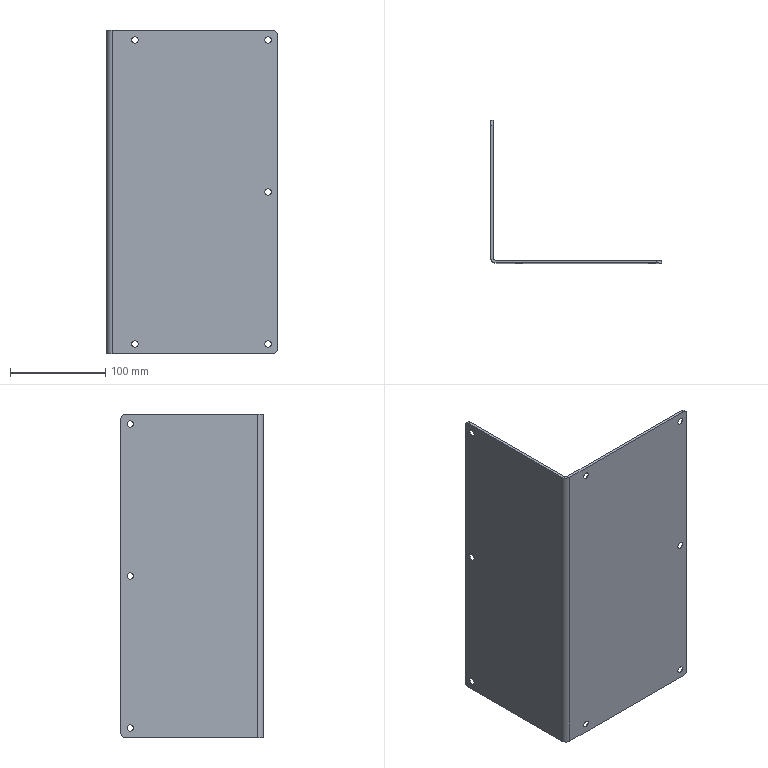Part | STEP file | PN_0001-12 Cover plate B | 1 solid | 30 faces | box 180 x 150 x 340 mm | volume 329639 mm3 | cone 16 | plane 8 | cylinder 6 | commonest cylinder face diameters 10 x4 6 x1 12 x1
STEP:
#1=CARTESIAN_POINT('',(0.,-10.,333.4));
#2=VERTEX_POINT('',#1);
#3=CARTESIAN_POINT('',(0.,-10.,326.6));
#4=VERTEX_POINT('',#3);
#5=CARTESIAN_POINT('',(0.,-10.,330.));
#6=DIRECTION('',(1.,0.,0.));
#7=DIRECTION('',(0.,1.,0.));
#8=AXIS2_PLACEMENT_3D('',#5,#6,#7);
#9=CIRCLE('',#8,3.4);
#10=EDGE_CURVE('',#2,#4,#9,.T.);
#11=ORIENTED_EDGE('',*,*,#10,.F.);
#12=CARTESIAN_POINT('',(3.,-10.,336.4));
#13=VERTEX_POINT('',#12);
#14=CARTESIAN_POINT('',(3.,-10.,336.4));
#15=DIRECTION('',(0.7071,0.,0.7071));
#16=VECTOR('',#15,1000.);
#17=LINE('',#14,#16);
#18=EDGE_CURVE('',#2,#13,#17,.T.);
#19=ORIENTED_EDGE('',*,*,#18,.T.);
#20=CARTESIAN_POINT('',(3.,-10.,323.6));
#21=VERTEX_POINT('',#20);
#22=CARTESIAN_POINT('',(3.,-10.,330.));
#23=DIRECTION('',(1.,0.,0.));
#24=DIRECTION('',(0.,0.,-1.));
#25=AXIS2_PLACEMENT_3D('',#22,#23,#24);
#26=CIRCLE('',#25,6.4);
#27=EDGE_CURVE('',#13,#21,#26,.T.);
#28=ORIENTED_EDGE('',*,*,#27,.T.);
#29=CARTESIAN_POINT('',(3.,-10.,323.6));
#30=DIRECTION('',(0.7071,0.,-0.7071));
#31=VECTOR('',#30,1000.);
#32=LINE('',#29,#31);
#33=EDGE_CURVE('',#4,#21,#32,.T.);
#34=ORIENTED_EDGE('',*,*,#33,.F.);
#35=EDGE_LOOP('',(#11,#19,#28,#34));
#36=FACE_OUTER_BOUND('',#35,.T.);
#37=CARTESIAN_POINT('',(3.,-10.,330.));
#38=DIRECTION('',(1.,0.,0.));
#39=DIRECTION('',(0.,0.,-1.));
#40=AXIS2_PLACEMENT_3D('',#37,#38,#39);
#41=CONICAL_SURFACE('',#40,6.4,0.7854);
#42=ADVANCED_FACE('',(#36),#41,.F.);
#43=CARTESIAN_POINT('',(0.,-10.,173.4));
#44=VERTEX_POINT('',#43);
#45=CARTESIAN_POINT('',(0.,-10.,166.6));
#46=VERTEX_POINT('',#45);
#47=CARTESIAN_POINT('',(0.,-10.,170.));
#48=DIRECTION('',(1.,0.,0.));
#49=DIRECTION('',(0.,1.,0.));
#50=AXIS2_PLACEMENT_3D('',#47,#48,#49);
#51=CIRCLE('',#50,3.4);
#52=EDGE_CURVE('',#44,#46,#51,.T.);
#53=ORIENTED_EDGE('',*,*,#52,.F.);
#54=CARTESIAN_POINT('',(3.,-10.,176.4));
#55=VERTEX_POINT('',#54);
#56=CARTESIAN_POINT('',(3.,-10.,176.4));
#57=DIRECTION('',(0.7071,0.,0.7071));
#58=VECTOR('',#57,1000.);
#59=LINE('',#56,#58);
#60=EDGE_CURVE('',#44,#55,#59,.T.);
#61=ORIENTED_EDGE('',*,*,#60,.T.);
#62=CARTESIAN_POINT('',(3.,-10.,163.6));
#63=VERTEX_POINT('',#62);
#64=CARTESIAN_POINT('',(3.,-10.,170.));
#65=DIRECTION('',(1.,0.,0.));
#66=DIRECTION('',(0.,0.,-1.));
#67=AXIS2_PLACEMENT_3D('',#64,#65,#66);
#68=CIRCLE('',#67,6.4);
#69=EDGE_CURVE('',#55,#63,#68,.T.);
#70=ORIENTED_EDGE('',*,*,#69,.T.);
#71=CARTESIAN_POINT('',(3.,-10.,163.6));
#72=DIRECTION('',(0.7071,0.,-0.7071));
#73=VECTOR('',#72,1000.);
#74=LINE('',#71,#73);
#75=EDGE_CURVE('',#46,#63,#74,.T.);
#76=ORIENTED_EDGE('',*,*,#75,.F.);
#77=EDGE_LOOP('',(#53,#61,#70,#76));
#78=FACE_OUTER_BOUND('',#77,.T.);
#79=CARTESIAN_POINT('',(3.,-10.,170.));
#80=DIRECTION('',(1.,0.,0.));
#81=DIRECTION('',(0.,0.,-1.));
#82=AXIS2_PLACEMENT_3D('',#79,#80,#81);
#83=CONICAL_SURFACE('',#82,6.4,0.7854);
#84=ADVANCED_FACE('',(#78),#83,.F.);
#85=CARTESIAN_POINT('',(0.,-10.,13.4));
#86=VERTEX_POINT('',#85);
#87=CARTESIAN_POINT('',(0.,-10.,6.6));
#88=VERTEX_POINT('',#87);
#89=CARTESIAN_POINT('',(0.,-10.,10.));
#90=DIRECTION('',(1.,0.,0.));
#91=DIRECTION('',(0.,1.,0.));
#92=AXIS2_PLACEMENT_3D('',#89,#90,#91);
#93=CIRCLE('',#92,3.4);
#94=EDGE_CURVE('',#86,#88,#93,.T.);
#95=ORIENTED_EDGE('',*,*,#94,.F.);
#96=CARTESIAN_POINT('',(3.,-10.,16.4));
#97=VERTEX_POINT('',#96);
#98=CARTESIAN_POINT('',(3.,-10.,16.4));
#99=DIRECTION('',(0.7071,0.,0.7071));
#100=VECTOR('',#99,1000.);
#101=LINE('',#98,#100);
#102=EDGE_CURVE('',#86,#97,#101,.T.);
#103=ORIENTED_EDGE('',*,*,#102,.T.);
#104=CARTESIAN_POINT('',(3.,-10.,3.6));
#105=VERTEX_POINT('',#104);
#106=CARTESIAN_POINT('',(3.,-10.,10.));
#107=DIRECTION('',(1.,0.,0.));
#108=DIRECTION('',(0.,0.,-1.));
#109=AXIS2_PLACEMENT_3D('',#106,#107,#108);
#110=CIRCLE('',#109,6.4);
#111=EDGE_CURVE('',#97,#105,#110,.T.);
#112=ORIENTED_EDGE('',*,*,#111,.T.);
#113=CARTESIAN_POINT('',(3.,-10.,3.6));
#114=DIRECTION('',(0.7071,0.,-0.7071));
#115=VECTOR('',#114,1000.);
#116=LINE('',#113,#115);
#117=EDGE_CURVE('',#88,#105,#116,.T.);
#118=ORIENTED_EDGE('',*,*,#117,.F.);
#119=EDGE_LOOP('',(#95,#103,#112,#118));
#120=FACE_OUTER_BOUND('',#119,.T.);
#121=CARTESIAN_POINT('',(3.,-10.,10.));
#122=DIRECTION('',(1.,0.,0.));
#123=DIRECTION('',(0.,0.,-1.));
#124=AXIS2_PLACEMENT_3D('',#121,#122,#123);
#125=CONICAL_SURFACE('',#124,6.4,0.7854);
#126=ADVANCED_FACE('',(#120),#125,.F.);
#127=CARTESIAN_POINT('',(30.,-150.,6.6));
#128=VERTEX_POINT('',#127);
#129=CARTESIAN_POINT('',(30.,-150.,13.4));
#130=VERTEX_POINT('',#129);
#131=CARTESIAN_POINT('',(30.,-150.,10.));
#132=DIRECTION('',(0.,1.,0.));
#133=DIRECTION('',(-1.,0.,0.));
#134=AXIS2_PLACEMENT_3D('',#131,#132,#133);
#135=CIRCLE('',#134,3.4);
#136=EDGE_CURVE('',#128,#130,#135,.T.);
#137=ORIENTED_EDGE('',*,*,#136,.F.);
#138=CARTESIAN_POINT('',(30.,-147.,3.6));
#139=VERTEX_POINT('',#138);
#140=CARTESIAN_POINT('',(30.,-147.,3.6));
#141=DIRECTION('',(0.,0.7071,-0.7071));
#142=VECTOR('',#141,1000.);
#143=LINE('',#140,#142);
#144=EDGE_CURVE('',#128,#139,#143,.T.);
#145=ORIENTED_EDGE('',*,*,#144,.T.);
#146=CARTESIAN_POINT('',(30.,-147.,16.4));
#147=VERTEX_POINT('',#146);
#148=CARTESIAN_POINT('',(30.,-147.,10.));
#149=DIRECTION('',(0.,1.,0.));
#150=DIRECTION('',(0.,0.,1.));
#151=AXIS2_PLACEMENT_3D('',#148,#149,#150);
#152=CIRCLE('',#151,6.4);
#153=EDGE_CURVE('',#139,#147,#152,.T.);
#154=ORIENTED_EDGE('',*,*,#153,.T.);
#155=CARTESIAN_POINT('',(30.,-147.,16.4));
#156=DIRECTION('',(0.,0.7071,0.7071));
#157=VECTOR('',#156,1000.);
#158=LINE('',#155,#157);
#159=EDGE_CURVE('',#130,#147,#158,.T.);
#160=ORIENTED_EDGE('',*,*,#159,.F.);
#161=EDGE_LOOP('',(#137,#145,#154,#160));
#162=FACE_OUTER_BOUND('',#161,.T.);
#163=CARTESIAN_POINT('',(30.,-147.,10.));
#164=DIRECTION('',(0.,1.,0.));
#165=DIRECTION('',(0.,0.,1.));
#166=AXIS2_PLACEMENT_3D('',#163,#164,#165);
#167=CONICAL_SURFACE('',#166,6.4,0.7854);
#168=ADVANCED_FACE('',(#162),#167,.F.);
#169=CARTESIAN_POINT('',(170.,-150.,6.6));
#170=VERTEX_POINT('',#169);
#171=CARTESIAN_POINT('',(170.,-150.,13.4));
#172=VERTEX_POINT('',#171);
#173=CARTESIAN_POINT('',(170.,-150.,10.));
#174=DIRECTION('',(0.,1.,0.));
#175=DIRECTION('',(-1.,0.,0.));
#176=AXIS2_PLACEMENT_3D('',#173,#174,#175);
#177=CIRCLE('',#176,3.4);
#178=EDGE_CURVE('',#170,#172,#177,.T.);
#179=ORIENTED_EDGE('',*,*,#178,.F.);
#180=CARTESIAN_POINT('',(170.,-147.,3.6));
#181=VERTEX_POINT('',#180);
#182=CARTESIAN_POINT('',(170.,-147.,3.6));
#183=DIRECTION('',(0.,0.7071,-0.7071));
#184=VECTOR('',#183,1000.);
#185=LINE('',#182,#184);
#186=EDGE_CURVE('',#170,#181,#185,.T.);
#187=ORIENTED_EDGE('',*,*,#186,.T.);
#188=CARTESIAN_POINT('',(170.,-147.,16.4));
#189=VERTEX_POINT('',#188);
#190=CARTESIAN_POINT('',(170.,-147.,10.));
#191=DIRECTION('',(0.,1.,0.));
#192=DIRECTION('',(0.,0.,1.));
#193=AXIS2_PLACEMENT_3D('',#190,#191,#192);
#194=CIRCLE('',#193,6.4);
#195=EDGE_CURVE('',#181,#189,#194,.T.);
#196=ORIENTED_EDGE('',*,*,#195,.T.);
#197=CARTESIAN_POINT('',(170.,-147.,16.4));
#198=DIRECTION('',(0.,0.7071,0.7071));
#199=VECTOR('',#198,1000.);
#200=LINE('',#197,#199);
#201=EDGE_CURVE('',#172,#189,#200,.T.);
#202=ORIENTED_EDGE('',*,*,#201,.F.);
#203=EDGE_LOOP('',(#179,#187,#196,#202));
#204=FACE_OUTER_BOUND('',#203,.T.);
#205=CARTESIAN_POINT('',(170.,-147.,10.));
#206=DIRECTION('',(0.,1.,0.));
#207=DIRECTION('',(0.,0.,1.));
#208=AXIS2_PLACEMENT_3D('',#205,#206,#207);
#209=CONICAL_SURFACE('',#208,6.4,0.7854);
#210=ADVANCED_FACE('',(#204),#209,.F.);
#211=CARTESIAN_POINT('',(170.,-150.,326.6));
#212=VERTEX_POINT('',#211);
#213=CARTESIAN_POINT('',(170.,-150.,333.4));
#214=VERTEX_POINT('',#213);
#215=CARTESIAN_POINT('',(170.,-150.,330.));
#216=DIRECTION('',(0.,1.,0.));
#217=DIRECTION('',(-1.,0.,0.));
#218=AXIS2_PLACEMENT_3D('',#215,#216,#217);
#219=CIRCLE('',#218,3.4);
#220=EDGE_CURVE('',#212,#214,#219,.T.);
#221=ORIENTED_EDGE('',*,*,#220,.F.);
#222=CARTESIAN_POINT('',(170.,-147.,323.6));
#223=VERTEX_POINT('',#222);
#224=CARTESIAN_POINT('',(170.,-147.,323.6));
#225=DIRECTION('',(0.,0.7071,-0.7071));
#226=VECTOR('',#225,1000.);
#227=LINE('',#224,#226);
#228=EDGE_CURVE('',#212,#223,#227,.T.);
#229=ORIENTED_EDGE('',*,*,#228,.T.);
#230=CARTESIAN_POINT('',(170.,-147.,336.4));
#231=VERTEX_POINT('',#230);
#232=CARTESIAN_POINT('',(170.,-147.,330.));
#233=DIRECTION('',(0.,1.,0.));
#234=DIRECTION('',(0.,0.,1.));
#235=AXIS2_PLACEMENT_3D('',#232,#233,#234);
#236=CIRCLE('',#235,6.4);
#237=EDGE_CURVE('',#223,#231,#236,.T.);
#238=ORIENTED_EDGE('',*,*,#237,.T.);
#239=CARTESIAN_POINT('',(170.,-147.,336.4));
#240=DIRECTION('',(0.,0.7071,0.7071));
#241=VECTOR('',#240,1000.);
#242=LINE('',#239,#241);
#243=EDGE_CURVE('',#214,#231,#242,.T.);
#244=ORIENTED_EDGE('',*,*,#243,.F.);
#245=EDGE_LOOP('',(#221,#229,#238,#244));
#246=FACE_OUTER_BOUND('',#245,.T.);
#247=CARTESIAN_POINT('',(170.,-147.,330.));
#248=DIRECTION('',(0.,1.,0.));
#249=DIRECTION('',(0.,0.,1.));
#250=AXIS2_PLACEMENT_3D('',#247,#248,#249);
#251=CONICAL_SURFACE('',#250,6.4,0.7854);
#252=ADVANCED_FACE('',(#246),#251,.F.);
#253=CARTESIAN_POINT('',(30.,-150.,326.6));
#254=VERTEX_POINT('',#253);
#255=CARTESIAN_POINT('',(30.,-150.,333.4));
#256=VERTEX_POINT('',#255);
#257=CARTESIAN_POINT('',(30.,-150.,330.));
#258=DIRECTION('',(0.,1.,0.));
#259=DIRECTION('',(-1.,0.,0.));
#260=AXIS2_PLACEMENT_3D('',#257,#258,#259);
#261=CIRCLE('',#260,3.4);
#262=EDGE_CURVE('',#254,#256,#261,.T.);
#263=ORIENTED_EDGE('',*,*,#262,.F.);
#264=CARTESIAN_POINT('',(30.,-147.,323.6));
#265=VERTEX_POINT('',#264);
#266=CARTESIAN_POINT('',(30.,-147.,323.6));
#267=DIRECTION('',(0.,0.7071,-0.7071));
#268=VECTOR('',#267,1000.);
#269=LINE('',#266,#268);
#270=EDGE_CURVE('',#254,#265,#269,.T.);
#271=ORIENTED_EDGE('',*,*,#270,.T.);
#272=CARTESIAN_POINT('',(30.,-147.,336.4));
#273=VERTEX_POINT('',#272);
#274=CARTESIAN_POINT('',(30.,-147.,330.));
#275=DIRECTION('',(0.,1.,0.));
#276=DIRECTION('',(0.,0.,1.));
#277=AXIS2_PLACEMENT_3D('',#274,#275,#276);
#278=CIRCLE('',#277,6.4);
#279=EDGE_CURVE('',#265,#273,#278,.T.);
#280=ORIENTED_EDGE('',*,*,#279,.T.);
#281=CARTESIAN_POINT('',(30.,-147.,336.4));
#282=DIRECTION('',(0.,0.7071,0.7071));
#283=VECTOR('',#282,1000.);
#284=LINE('',#281,#283);
#285=EDGE_CURVE('',#256,#273,#284,.T.);
#286=ORIENTED_EDGE('',*,*,#285,.F.);
#287=EDGE_LOOP('',(#263,#271,#280,#286));
#288=FACE_OUTER_BOUND('',#287,.T.);
#289=CARTESIAN_POINT('',(30.,-147.,330.));
#290=DIRECTION('',(0.,1.,0.));
#291=DIRECTION('',(0.,0.,1.));
#292=AXIS2_PLACEMENT_3D('',#289,#290,#291);
#293=CONICAL_SURFACE('',#292,6.4,0.7854);
#294=ADVANCED_FACE('',(#288),#293,.F.);
#295=CARTESIAN_POINT('',(170.,-150.,166.6));
#296=VERTEX_POINT('',#295);
#297=CARTESIAN_POINT('',(170.,-150.,173.4));
#298=VERTEX_POINT('',#297);
#299=CARTESIAN_POINT('',(170.,-150.,170.));
#300=DIRECTION('',(0.,1.,0.));
#301=DIRECTION('',(-1.,0.,0.));
#302=AXIS2_PLACEMENT_3D('',#299,#300,#301);
#303=CIRCLE('',#302,3.4);
#304=EDGE_CURVE('',#296,#298,#303,.T.);
#305=ORIENTED_EDGE('',*,*,#304,.F.);
#306=CARTESIAN_POINT('',(170.,-147.,163.6));
#307=VERTEX_POINT('',#306);
#308=CARTESIAN_POINT('',(170.,-147.,163.6));
#309=DIRECTION('',(0.,0.7071,-0.7071));
#310=VECTOR('',#309,1000.);
#311=LINE('',#308,#310);
#312=EDGE_CURVE('',#296,#307,#311,.T.);
#313=ORIENTED_EDGE('',*,*,#312,.T.);
#314=CARTESIAN_POINT('',(170.,-147.,176.4));
#315=VERTEX_POINT('',#314);
#316=CARTESIAN_POINT('',(170.,-147.,170.));
#317=DIRECTION('',(0.,1.,0.));
#318=DIRECTION('',(0.,0.,1.));
#319=AXIS2_PLACEMENT_3D('',#316,#317,#318);
#320=CIRCLE('',#319,6.4);
#321=EDGE_CURVE('',#307,#315,#320,.T.);
#322=ORIENTED_EDGE('',*,*,#321,.T.);
#323=CARTESIAN_POINT('',(170.,-147.,176.4));
#324=DIRECTION('',(0.,0.7071,0.7071));
#325=VECTOR('',#324,1000.);
#326=LINE('',#323,#325);
#327=EDGE_CURVE('',#298,#315,#326,.T.);
#328=ORIENTED_EDGE('',*,*,#327,.F.);
#329=EDGE_LOOP('',(#305,#313,#322,#328));
#330=FACE_OUTER_BOUND('',#329,.T.);
#331=CARTESIAN_POINT('',(170.,-147.,170.));
#332=DIRECTION('',(0.,1.,0.));
#333=DIRECTION('',(0.,0.,1.));
#334=AXIS2_PLACEMENT_3D('',#331,#332,#333);
#335=CONICAL_SURFACE('',#334,6.4,0.7854);
#336=ADVANCED_FACE('',(#330),#335,.F.);
#337=CARTESIAN_POINT('',(3.,-10.,330.));
#338=DIRECTION('',(1.,0.,0.));
#339=DIRECTION('',(0.,0.,-1.));
#340=AXIS2_PLACEMENT_3D('',#337,#338,#339);
#341=CIRCLE('',#340,6.4);
#342=EDGE_CURVE('',#21,#13,#341,.T.);
#343=ORIENTED_EDGE('',*,*,#342,.F.);
#344=ORIENTED_EDGE('',*,*,#27,.F.);
#345=EDGE_LOOP('',(#343,#344));
#346=FACE_BOUND('',#345,.T.);
#347=CARTESIAN_POINT('',(3.,-10.,170.));
#348=DIRECTION('',(1.,0.,0.));
#349=DIRECTION('',(0.,0.,-1.));
#350=AXIS2_PLACEMENT_3D('',#347,#348,#349);
#351=CIRCLE('',#350,6.4);
#352=EDGE_CURVE('',#63,#55,#351,.T.);
#353=ORIENTED_EDGE('',*,*,#352,.F.);
#354=ORIENTED_EDGE('',*,*,#69,.F.);
#355=EDGE_LOOP('',(#353,#354));
#356=FACE_BOUND('',#355,.T.);
#357=CARTESIAN_POINT('',(3.,-144.,0.));
#358=VERTEX_POINT('',#357);
#359=CARTESIAN_POINT('',(3.,-5.,0.));
#360=VERTEX_POINT('',#359);
#361=CARTESIAN_POINT('',(3.,-144.,0.));
#362=DIRECTION('',(0.,1.,0.));
#363=VECTOR('',#362,1000.);
#364=LINE('',#361,#363);
#365=EDGE_CURVE('',#358,#360,#364,.T.);
#366=ORIENTED_EDGE('',*,*,#365,.T.);
#367=CARTESIAN_POINT('',(3.,0.,5.));
#368=VERTEX_POINT('',#367);
#369=CARTESIAN_POINT('',(3.,-5.,5.));
#370=DIRECTION('',(1.,0.,0.));
#371=DIRECTION('',(0.,-1.,0.));
#372=AXIS2_PLACEMENT_3D('',#369,#370,#371);
#373=CIRCLE('',#372,5.);
#374=EDGE_CURVE('',#360,#368,#373,.T.);
#375=ORIENTED_EDGE('',*,*,#374,.T.);
#376=CARTESIAN_POINT('',(3.,0.,335.));
#377=VERTEX_POINT('',#376);
#378=CARTESIAN_POINT('',(3.,0.,340.));
#379=DIRECTION('',(0.,0.,-1.));
#380=VECTOR('',#379,1000.);
#381=LINE('',#378,#380);
#382=EDGE_CURVE('',#377,#368,#381,.T.);
#383=ORIENTED_EDGE('',*,*,#382,.F.);
#384=CARTESIAN_POINT('',(3.,-5.,340.));
#385=VERTEX_POINT('',#384);
#386=CARTESIAN_POINT('',(3.,-5.,335.));
#387=DIRECTION('',(1.,0.,0.));
#388=DIRECTION('',(0.,-1.,0.));
#389=AXIS2_PLACEMENT_3D('',#386,#387,#388);
#390=CIRCLE('',#389,5.);
#391=EDGE_CURVE('',#377,#385,#390,.T.);
#392=ORIENTED_EDGE('',*,*,#391,.T.);
#393=CARTESIAN_POINT('',(3.,-144.,340.));
#394=VERTEX_POINT('',#393);
#395=CARTESIAN_POINT('',(3.,-144.,340.));
#396=DIRECTION('',(0.,1.,0.));
#397=VECTOR('',#396,1000.);
#398=LINE('',#395,#397);
#399=EDGE_CURVE('',#394,#385,#398,.T.);
#400=ORIENTED_EDGE('',*,*,#399,.F.);
#401=CARTESIAN_POINT('',(3.,-144.,340.));
#402=DIRECTION('',(0.,0.,-1.));
#403=VECTOR('',#402,1000.);
#404=LINE('',#401,#403);
#405=EDGE_CURVE('',#394,#358,#404,.T.);
#406=ORIENTED_EDGE('',*,*,#405,.T.);
#407=EDGE_LOOP('',(#366,#375,#383,#392,#400,#406));
#408=FACE_OUTER_BOUND('',#407,.T.);
#409=CARTESIAN_POINT('',(3.,-10.,10.));
#410=DIRECTION('',(1.,0.,0.));
#411=DIRECTION('',(0.,0.,-1.));
#412=AXIS2_PLACEMENT_3D('',#409,#410,#411);
#413=CIRCLE('',#412,6.4);
#414=EDGE_CURVE('',#105,#97,#413,.T.);
#415=ORIENTED_EDGE('',*,*,#414,.F.);
#416=ORIENTED_EDGE('',*,*,#111,.F.);
#417=EDGE_LOOP('',(#415,#416));
#418=FACE_BOUND('',#417,.T.);
#419=CARTESIAN_POINT('',(3.,-144.,340.));
#420=DIRECTION('',(-1.,0.,0.));
#421=DIRECTION('',(0.,-1.,0.));
#422=AXIS2_PLACEMENT_3D('',#419,#420,#421);
#423=PLANE('',#422);
#424=ADVANCED_FACE('',(#346,#356,#408,#418),#423,.F.);
#425=ORIENTED_EDGE('',*,*,#382,.T.);
#426=CARTESIAN_POINT('',(0.,0.,5.));
#427=VERTEX_POINT('',#426);
#428=CARTESIAN_POINT('',(3.,0.,5.));
#429=DIRECTION('',(-1.,0.,0.));
#430=VECTOR('',#429,1000.);
#431=LINE('',#428,#430);
#432=EDGE_CURVE('',#368,#427,#431,.T.);
#433=ORIENTED_EDGE('',*,*,#432,.T.);
#434=CARTESIAN_POINT('',(0.,0.,335.));
#435=VERTEX_POINT('',#434);
#436=CARTESIAN_POINT('',(0.,0.,340.));
#437=DIRECTION('',(0.,0.,-1.));
#438=VECTOR('',#437,1000.);
#439=LINE('',#436,#438);
#440=EDGE_CURVE('',#435,#427,#439,.T.);
#441=ORIENTED_EDGE('',*,*,#440,.F.);
#442=CARTESIAN_POINT('',(3.,0.,335.));
#443=DIRECTION('',(1.,0.,0.));
#444=VECTOR('',#443,1000.);
#445=LINE('',#442,#444);
#446=EDGE_CURVE('',#435,#377,#445,.T.);
#447=ORIENTED_EDGE('',*,*,#446,.T.);
#448=EDGE_LOOP('',(#425,#433,#441,#447));
#449=FACE_OUTER_BOUND('',#448,.T.);
#450=CARTESIAN_POINT('',(3.,0.,340.));
#451=DIRECTION('',(0.,-1.,0.));
#452=DIRECTION('',(0.,0.,-1.));
#453=AXIS2_PLACEMENT_3D('',#450,#451,#452);
#454=PLANE('',#453);
#455=ADVANCED_FACE('',(#449),#454,.F.);
#456=CARTESIAN_POINT('',(0.,-10.,330.));
#457=DIRECTION('',(1.,0.,0.));
#458=DIRECTION('',(0.,1.,0.));
#459=AXIS2_PLACEMENT_3D('',#456,#457,#458);
#460=CIRCLE('',#459,3.4);
#461=EDGE_CURVE('',#4,#2,#460,.T.);
#462=ORIENTED_EDGE('',*,*,#461,.T.);
#463=ORIENTED_EDGE('',*,*,#10,.T.);
#464=EDGE_LOOP('',(#462,#463));
#465=FACE_BOUND('',#464,.T.);
#466=CARTESIAN_POINT('',(0.,-10.,170.));
#467=DIRECTION('',(1.,0.,0.));
#468=DIRECTION('',(0.,1.,0.));
#469=AXIS2_PLACEMENT_3D('',#466,#467,#468);
#470=CIRCLE('',#469,3.4);
#471=EDGE_CURVE('',#46,#44,#470,.T.);
#472=ORIENTED_EDGE('',*,*,#471,.T.);
#473=ORIENTED_EDGE('',*,*,#52,.T.);
#474=EDGE_LOOP('',(#472,#473));
#475=FACE_BOUND('',#474,.T.);
#476=CARTESIAN_POINT('',(0.,-10.,10.));
#477=DIRECTION('',(1.,0.,0.));
#478=DIRECTION('',(0.,1.,0.));
#479=AXIS2_PLACEMENT_3D('',#476,#477,#478);
#480=CIRCLE('',#479,3.4);
#481=EDGE_CURVE('',#88,#86,#480,.T.);
#482=ORIENTED_EDGE('',*,*,#481,.T.);
#483=ORIENTED_EDGE('',*,*,#94,.T.);
#484=EDGE_LOOP('',(#482,#483));
#485=FACE_BOUND('',#484,.T.);
#486=ORIENTED_EDGE('',*,*,#440,.T.);
#487=CARTESIAN_POINT('',(0.,-5.,0.));
#488=VERTEX_POINT('',#487);
#489=CARTESIAN_POINT('',(0.,-5.,5.));
#490=DIRECTION('',(-1.,0.,0.));
#491=DIRECTION('',(0.,1.,0.));
#492=AXIS2_PLACEMENT_3D('',#489,#490,#491);
#493=CIRCLE('',#492,5.);
#494=EDGE_CURVE('',#427,#488,#493,.T.);
#495=ORIENTED_EDGE('',*,*,#494,.T.);
#496=CARTESIAN_POINT('',(0.,-144.,0.));
#497=VERTEX_POINT('',#496);
#498=CARTESIAN_POINT('',(0.,0.,0.));
#499=DIRECTION('',(0.,-1.,0.));
#500=VECTOR('',#499,1000.);
#501=LINE('',#498,#500);
#502=EDGE_CURVE('',#488,#497,#501,.T.);
#503=ORIENTED_EDGE('',*,*,#502,.T.);
#504=CARTESIAN_POINT('',(0.,-144.,340.));
#505=VERTEX_POINT('',#504);
#506=CARTESIAN_POINT('',(0.,-144.,340.));
#507=DIRECTION('',(0.,0.,-1.));
#508=VECTOR('',#507,1000.);
#509=LINE('',#506,#508);
#510=EDGE_CURVE('',#505,#497,#509,.T.);
#511=ORIENTED_EDGE('',*,*,#510,.F.);
#512=CARTESIAN_POINT('',(0.,-5.,340.));
#513=VERTEX_POINT('',#512);
#514=CARTESIAN_POINT('',(0.,0.,340.));
#515=DIRECTION('',(0.,-1.,0.));
#516=VECTOR('',#515,1000.);
#517=LINE('',#514,#516);
#518=EDGE_CURVE('',#513,#505,#517,.T.);
#519=ORIENTED_EDGE('',*,*,#518,.F.);
#520=CARTESIAN_POINT('',(0.,-5.,335.));
#521=DIRECTION('',(-1.,0.,0.));
#522=DIRECTION('',(0.,1.,0.));
#523=AXIS2_PLACEMENT_3D('',#520,#521,#522);
#524=CIRCLE('',#523,5.);
#525=EDGE_CURVE('',#513,#435,#524,.T.);
#526=ORIENTED_EDGE('',*,*,#525,.T.);
#527=EDGE_LOOP('',(#486,#495,#503,#511,#519,#526));
#528=FACE_OUTER_BOUND('',#527,.T.);
#529=CARTESIAN_POINT('',(0.,0.,340.));
#530=DIRECTION('',(1.,0.,0.));
#531=DIRECTION('',(0.,1.,0.));
#532=AXIS2_PLACEMENT_3D('',#529,#530,#531);
#533=PLANE('',#532);
#534=ADVANCED_FACE('',(#465,#475,#485,#528),#533,.F.);
#535=CARTESIAN_POINT('',(6.,-150.,0.));
#536=VERTEX_POINT('',#535);
#537=CARTESIAN_POINT('',(6.,-144.,0.));
#538=DIRECTION('',(0.,0.,1.));
#539=DIRECTION('',(1.,0.,0.));
#540=AXIS2_PLACEMENT_3D('',#537,#538,#539);
#541=CIRCLE('',#540,6.);
#542=EDGE_CURVE('',#497,#536,#541,.T.);
#543=ORIENTED_EDGE('',*,*,#542,.T.);
#544=CARTESIAN_POINT('',(6.,-150.,340.));
#545=VERTEX_POINT('',#544);
#546=CARTESIAN_POINT('',(6.,-150.,340.));
#547=DIRECTION('',(0.,0.,-1.));
#548=VECTOR('',#547,1000.);
#549=LINE('',#546,#548);
#550=EDGE_CURVE('',#545,#536,#549,.T.);
#551=ORIENTED_EDGE('',*,*,#550,.F.);
#552=CARTESIAN_POINT('',(6.,-144.,340.));
#553=DIRECTION('',(0.,0.,1.));
#554=DIRECTION('',(1.,0.,0.));
#555=AXIS2_PLACEMENT_3D('',#552,#553,#554);
#556=CIRCLE('',#555,6.);
#557=EDGE_CURVE('',#505,#545,#556,.T.);
#558=ORIENTED_EDGE('',*,*,#557,.F.);
#559=ORIENTED_EDGE('',*,*,#510,.T.);
#560=EDGE_LOOP('',(#543,#551,#558,#559));
#561=FACE_OUTER_BOUND('',#560,.T.);
#562=CARTESIAN_POINT('',(6.,-144.,340.));
#563=DIRECTION('',(0.,0.,-1.));
#564=DIRECTION('',(-1.,0.,0.));
#565=AXIS2_PLACEMENT_3D('',#562,#563,#564);
#566=CYLINDRICAL_SURFACE('',#565,6.);
#567=ADVANCED_FACE('',(#561),#566,.T.);
#568=CARTESIAN_POINT('',(30.,-150.,10.));
#569=DIRECTION('',(0.,1.,0.));
#570=DIRECTION('',(-1.,0.,0.));
#571=AXIS2_PLACEMENT_3D('',#568,#569,#570);
#572=CIRCLE('',#571,3.4);
#573=EDGE_CURVE('',#130,#128,#572,.T.);
#574=ORIENTED_EDGE('',*,*,#573,.T.);
#575=ORIENTED_EDGE('',*,*,#136,.T.);
#576=EDGE_LOOP('',(#574,#575));
#577=FACE_BOUND('',#576,.T.);
#578=CARTESIAN_POINT('',(170.,-150.,10.));
#579=DIRECTION('',(0.,1.,0.));
#580=DIRECTION('',(-1.,0.,0.));
#581=AXIS2_PLACEMENT_3D('',#578,#579,#580);
#582=CIRCLE('',#581,3.4);
#583=EDGE_CURVE('',#172,#170,#582,.T.);
#584=ORIENTED_EDGE('',*,*,#583,.T.);
#585=ORIENTED_EDGE('',*,*,#178,.T.);
#586=EDGE_LOOP('',(#584,#585));
#587=FACE_BOUND('',#586,.T.);
#588=CARTESIAN_POINT('',(170.,-150.,330.));
#589=DIRECTION('',(0.,1.,0.));
#590=DIRECTION('',(-1.,0.,0.));
#591=AXIS2_PLACEMENT_3D('',#588,#589,#590);
#592=CIRCLE('',#591,3.4);
#593=EDGE_CURVE('',#214,#212,#592,.T.);
#594=ORIENTED_EDGE('',*,*,#593,.T.);
#595=ORIENTED_EDGE('',*,*,#220,.T.);
#596=EDGE_LOOP('',(#594,#595));
#597=FACE_BOUND('',#596,.T.);
#598=CARTESIAN_POINT('',(30.,-150.,330.));
#599=DIRECTION('',(0.,1.,0.));
#600=DIRECTION('',(-1.,0.,0.));
#601=AXIS2_PLACEMENT_3D('',#598,#599,#600);
#602=CIRCLE('',#601,3.4);
#603=EDGE_CURVE('',#256,#254,#602,.T.);
#604=ORIENTED_EDGE('',*,*,#603,.T.);
#605=ORIENTED_EDGE('',*,*,#262,.T.);
#606=EDGE_LOOP('',(#604,#605));
#607=FACE_BOUND('',#606,.T.);
#608=CARTESIAN_POINT('',(170.,-150.,170.));
#609=DIRECTION('',(0.,1.,0.));
#610=DIRECTION('',(-1.,0.,0.));
#611=AXIS2_PLACEMENT_3D('',#608,#609,#610);
#612=CIRCLE('',#611,3.4);
#613=EDGE_CURVE('',#298,#296,#612,.T.);
#614=ORIENTED_EDGE('',*,*,#613,.T.);
#615=ORIENTED_EDGE('',*,*,#304,.T.);
#616=EDGE_LOOP('',(#614,#615));
#617=FACE_BOUND('',#616,.T.);
#618=CARTESIAN_POINT('',(175.,-150.,0.));
#619=VERTEX_POINT('',#618);
#620=CARTESIAN_POINT('',(6.,-150.,0.));
#621=DIRECTION('',(1.,0.,0.));
#622=VECTOR('',#621,1000.);
#623=LINE('',#620,#622);
#624=EDGE_CURVE('',#536,#619,#623,.T.);
#625=ORIENTED_EDGE('',*,*,#624,.T.);
#626=CARTESIAN_POINT('',(180.,-150.,5.));
#627=VERTEX_POINT('',#626);
#628=CARTESIAN_POINT('',(175.,-150.,5.));
#629=DIRECTION('',(0.,-1.,0.));
#630=DIRECTION('',(-1.,0.,0.));
#631=AXIS2_PLACEMENT_3D('',#628,#629,#630);
#632=CIRCLE('',#631,5.);
#633=EDGE_CURVE('',#619,#627,#632,.T.);
#634=ORIENTED_EDGE('',*,*,#633,.T.);
#635=CARTESIAN_POINT('',(180.,-150.,335.));
#636=VERTEX_POINT('',#635);
#637=CARTESIAN_POINT('',(180.,-150.,340.));
#638=DIRECTION('',(0.,0.,-1.));
#639=VECTOR('',#638,1000.);
#640=LINE('',#637,#639);
#641=EDGE_CURVE('',#636,#627,#640,.T.);
#642=ORIENTED_EDGE('',*,*,#641,.F.);
#643=CARTESIAN_POINT('',(175.,-150.,340.));
#644=VERTEX_POINT('',#643);
#645=CARTESIAN_POINT('',(175.,-150.,335.));
#646=DIRECTION('',(0.,-1.,0.));
#647=DIRECTION('',(-1.,0.,0.));
#648=AXIS2_PLACEMENT_3D('',#645,#646,#647);
#649=CIRCLE('',#648,5.);
#650=EDGE_CURVE('',#636,#644,#649,.T.);
#651=ORIENTED_EDGE('',*,*,#650,.T.);
#652=CARTESIAN_POINT('',(6.,-150.,340.));
#653=DIRECTION('',(1.,0.,0.));
#654=VECTOR('',#653,1000.);
#655=LINE('',#652,#654);
#656=EDGE_CURVE('',#545,#644,#655,.T.);
#657=ORIENTED_EDGE('',*,*,#656,.F.);
#658=ORIENTED_EDGE('',*,*,#550,.T.);
#659=EDGE_LOOP('',(#625,#634,#642,#651,#657,#658));
#660=FACE_OUTER_BOUND('',#659,.T.);
#661=CARTESIAN_POINT('',(6.,-150.,340.));
#662=DIRECTION('',(0.,1.,0.));
#663=DIRECTION('',(-1.,0.,0.));
#664=AXIS2_PLACEMENT_3D('',#661,#662,#663);
#665=PLANE('',#664);
#666=ADVANCED_FACE('',(#577,#587,#597,#607,#617,#660),#665,.F.);
#667=ORIENTED_EDGE('',*,*,#641,.T.);
#668=CARTESIAN_POINT('',(180.,-147.,5.));
#669=VERTEX_POINT('',#668);
#670=CARTESIAN_POINT('',(180.,-150.,5.));
#671=DIRECTION('',(0.,1.,0.));
#672=VECTOR('',#671,1000.);
#673=LINE('',#670,#672);
#674=EDGE_CURVE('',#627,#669,#673,.T.);
#675=ORIENTED_EDGE('',*,*,#674,.T.);
#676=CARTESIAN_POINT('',(180.,-147.,335.));
#677=VERTEX_POINT('',#676);
#678=CARTESIAN_POINT('',(180.,-147.,340.));
#679=DIRECTION('',(0.,0.,-1.));
#680=VECTOR('',#679,1000.);
#681=LINE('',#678,#680);
#682=EDGE_CURVE('',#677,#669,#681,.T.);
#683=ORIENTED_EDGE('',*,*,#682,.F.);
#684=CARTESIAN_POINT('',(180.,-150.,335.));
#685=DIRECTION('',(0.,-1.,0.));
#686=VECTOR('',#685,1000.);
#687=LINE('',#684,#686);
#688=EDGE_CURVE('',#677,#636,#687,.T.);
#689=ORIENTED_EDGE('',*,*,#688,.T.);
#690=EDGE_LOOP('',(#667,#675,#683,#689));
#691=FACE_OUTER_BOUND('',#690,.T.);
#692=CARTESIAN_POINT('',(180.,-150.,340.));
#693=DIRECTION('',(-1.,0.,0.));
#694=DIRECTION('',(0.,0.,1.));
#695=AXIS2_PLACEMENT_3D('',#692,#693,#694);
#696=PLANE('',#695);
#697=ADVANCED_FACE('',(#691),#696,.F.);
#698=CARTESIAN_POINT('',(30.,-147.,10.));
#699=DIRECTION('',(0.,1.,0.));
#700=DIRECTION('',(0.,0.,1.));
#701=AXIS2_PLACEMENT_3D('',#698,#699,#700);
#702=CIRCLE('',#701,6.4);
#703=EDGE_CURVE('',#147,#139,#702,.T.);
#704=ORIENTED_EDGE('',*,*,#703,.F.);
#705=ORIENTED_EDGE('',*,*,#153,.F.);
#706=EDGE_LOOP('',(#704,#705));
#707=FACE_BOUND('',#706,.T.);
#708=CARTESIAN_POINT('',(170.,-147.,10.));
#709=DIRECTION('',(0.,1.,0.));
#710=DIRECTION('',(0.,0.,1.));
#711=AXIS2_PLACEMENT_3D('',#708,#709,#710);
#712=CIRCLE('',#711,6.4);
#713=EDGE_CURVE('',#189,#181,#712,.T.);
#714=ORIENTED_EDGE('',*,*,#713,.F.);
#715=ORIENTED_EDGE('',*,*,#195,.F.);
#716=EDGE_LOOP('',(#714,#715));
#717=FACE_BOUND('',#716,.T.);
#718=CARTESIAN_POINT('',(170.,-147.,330.));
#719=DIRECTION('',(0.,1.,0.));
#720=DIRECTION('',(0.,0.,1.));
#721=AXIS2_PLACEMENT_3D('',#718,#719,#720);
#722=CIRCLE('',#721,6.4);
#723=EDGE_CURVE('',#231,#223,#722,.T.);
#724=ORIENTED_EDGE('',*,*,#723,.F.);
#725=ORIENTED_EDGE('',*,*,#237,.F.);
#726=EDGE_LOOP('',(#724,#725));
#727=FACE_BOUND('',#726,.T.);
#728=CARTESIAN_POINT('',(30.,-147.,330.));
#729=DIRECTION('',(0.,1.,0.));
#730=DIRECTION('',(0.,0.,1.));
#731=AXIS2_PLACEMENT_3D('',#728,#729,#730);
#732=CIRCLE('',#731,6.4);
#733=EDGE_CURVE('',#273,#265,#732,.T.);
#734=ORIENTED_EDGE('',*,*,#733,.F.);
#735=ORIENTED_EDGE('',*,*,#279,.F.);
#736=EDGE_LOOP('',(#734,#735));
#737=FACE_BOUND('',#736,.T.);
#738=CARTESIAN_POINT('',(170.,-147.,170.));
#739=DIRECTION('',(0.,1.,0.));
#740=DIRECTION('',(0.,0.,1.));
#741=AXIS2_PLACEMENT_3D('',#738,#739,#740);
#742=CIRCLE('',#741,6.4);
#743=EDGE_CURVE('',#315,#307,#742,.T.);
#744=ORIENTED_EDGE('',*,*,#743,.F.);
#745=ORIENTED_EDGE('',*,*,#321,.F.);
#746=EDGE_LOOP('',(#744,#745));
#747=FACE_BOUND('',#746,.T.);
#748=ORIENTED_EDGE('',*,*,#682,.T.);
#749=CARTESIAN_POINT('',(175.,-147.,0.));
#750=VERTEX_POINT('',#749);
#751=CARTESIAN_POINT('',(175.,-147.,5.));
#752=DIRECTION('',(0.,1.,0.));
#753=DIRECTION('',(1.,0.,0.));
#754=AXIS2_PLACEMENT_3D('',#751,#752,#753);
#755=CIRCLE('',#754,5.);
#756=EDGE_CURVE('',#669,#750,#755,.T.);
#757=ORIENTED_EDGE('',*,*,#756,.T.);
#758=CARTESIAN_POINT('',(6.,-147.,0.));
#759=VERTEX_POINT('',#758);
#760=CARTESIAN_POINT('',(180.,-147.,0.));
#761=DIRECTION('',(-1.,0.,0.));
#762=VECTOR('',#761,1000.);
#763=LINE('',#760,#762);
#764=EDGE_CURVE('',#750,#759,#763,.T.);
#765=ORIENTED_EDGE('',*,*,#764,.T.);
#766=CARTESIAN_POINT('',(6.,-147.,340.));
#767=VERTEX_POINT('',#766);
#768=CARTESIAN_POINT('',(6.,-147.,340.));
#769=DIRECTION('',(0.,0.,-1.));
#770=VECTOR('',#769,1000.);
#771=LINE('',#768,#770);
#772=EDGE_CURVE('',#767,#759,#771,.T.);
#773=ORIENTED_EDGE('',*,*,#772,.F.);
#774=CARTESIAN_POINT('',(175.,-147.,340.));
#775=VERTEX_POINT('',#774);
#776=CARTESIAN_POINT('',(180.,-147.,340.));
#777=DIRECTION('',(-1.,0.,0.));
#778=VECTOR('',#777,1000.);
#779=LINE('',#776,#778);
#780=EDGE_CURVE('',#775,#767,#779,.T.);
#781=ORIENTED_EDGE('',*,*,#780,.F.);
#782=CARTESIAN_POINT('',(175.,-147.,335.));
#783=DIRECTION('',(0.,1.,0.));
#784=DIRECTION('',(1.,0.,0.));
#785=AXIS2_PLACEMENT_3D('',#782,#783,#784);
#786=CIRCLE('',#785,5.);
#787=EDGE_CURVE('',#775,#677,#786,.T.);
#788=ORIENTED_EDGE('',*,*,#787,.T.);
#789=EDGE_LOOP('',(#748,#757,#765,#773,#781,#788));
#790=FACE_OUTER_BOUND('',#789,.T.);
#791=CARTESIAN_POINT('',(180.,-147.,340.));
#792=DIRECTION('',(0.,-1.,0.));
#793=DIRECTION('',(1.,0.,0.));
#794=AXIS2_PLACEMENT_3D('',#791,#792,#793);
#795=PLANE('',#794);
#796=ADVANCED_FACE('',(#707,#717,#727,#737,#747,#790),#795,.F.);
#797=CARTESIAN_POINT('',(6.,-144.,0.));
#798=DIRECTION('',(0.,0.,-1.));
#799=DIRECTION('',(-1.,0.,0.));
#800=AXIS2_PLACEMENT_3D('',#797,#798,#799);
#801=CIRCLE('',#800,3.);
#802=EDGE_CURVE('',#759,#358,#801,.T.);
#803=ORIENTED_EDGE('',*,*,#802,.T.);
#804=ORIENTED_EDGE('',*,*,#405,.F.);
#805=CARTESIAN_POINT('',(6.,-144.,340.));
#806=DIRECTION('',(0.,0.,-1.));
#807=DIRECTION('',(-1.,0.,0.));
#808=AXIS2_PLACEMENT_3D('',#805,#806,#807);
#809=CIRCLE('',#808,3.);
#810=EDGE_CURVE('',#767,#394,#809,.T.);
#811=ORIENTED_EDGE('',*,*,#810,.F.);
#812=ORIENTED_EDGE('',*,*,#772,.T.);
#813=EDGE_LOOP('',(#803,#804,#811,#812));
#814=FACE_OUTER_BOUND('',#813,.T.);
#815=CARTESIAN_POINT('',(6.,-144.,340.));
#816=DIRECTION('',(0.,0.,-1.));
#817=DIRECTION('',(-1.,0.,0.));
#818=AXIS2_PLACEMENT_3D('',#815,#816,#817);
#819=CYLINDRICAL_SURFACE('',#818,3.);
#820=ADVANCED_FACE('',(#814),#819,.F.);
#821=ORIENTED_EDGE('',*,*,#656,.T.);
#822=CARTESIAN_POINT('',(175.,-147.,340.));
#823=DIRECTION('',(0.,1.,0.));
#824=VECTOR('',#823,1000.);
#825=LINE('',#822,#824);
#826=EDGE_CURVE('',#644,#775,#825,.T.);
#827=ORIENTED_EDGE('',*,*,#826,.T.);
#828=ORIENTED_EDGE('',*,*,#780,.T.);
#829=ORIENTED_EDGE('',*,*,#810,.T.);
#830=ORIENTED_EDGE('',*,*,#399,.T.);
#831=CARTESIAN_POINT('',(0.,-5.,340.));
#832=DIRECTION('',(-1.,0.,0.));
#833=VECTOR('',#832,1000.);
#834=LINE('',#831,#833);
#835=EDGE_CURVE('',#385,#513,#834,.T.);
#836=ORIENTED_EDGE('',*,*,#835,.T.);
#837=ORIENTED_EDGE('',*,*,#518,.T.);
#838=ORIENTED_EDGE('',*,*,#557,.T.);
#839=EDGE_LOOP('',(#821,#827,#828,#829,#830,#836,#837,#838));
#840=FACE_OUTER_BOUND('',#839,.T.);
#841=CARTESIAN_POINT('',(6.,-144.,340.));
#842=DIRECTION('',(0.,0.,1.));
#843=DIRECTION('',(1.,0.,0.));
#844=AXIS2_PLACEMENT_3D('',#841,#842,#843);
#845=PLANE('',#844);
#846=ADVANCED_FACE('',(#840),#845,.T.);
#847=ORIENTED_EDGE('',*,*,#764,.F.);
#848=CARTESIAN_POINT('',(175.,-144.,0.));
#849=DIRECTION('',(0.,-1.,0.));
#850=VECTOR('',#849,1000.);
#851=LINE('',#848,#850);
#852=EDGE_CURVE('',#750,#619,#851,.T.);
#853=ORIENTED_EDGE('',*,*,#852,.T.);
#854=ORIENTED_EDGE('',*,*,#624,.F.);
#855=ORIENTED_EDGE('',*,*,#542,.F.);
#856=ORIENTED_EDGE('',*,*,#502,.F.);
#857=CARTESIAN_POINT('',(6.,-5.,0.));
#858=DIRECTION('',(1.,0.,0.));
#859=VECTOR('',#858,1000.);
#860=LINE('',#857,#859);
#861=EDGE_CURVE('',#488,#360,#860,.T.);
#862=ORIENTED_EDGE('',*,*,#861,.T.);
#863=ORIENTED_EDGE('',*,*,#365,.F.);
#864=ORIENTED_EDGE('',*,*,#802,.F.);
#865=EDGE_LOOP('',(#847,#853,#854,#855,#856,#862,#863,#864));
#866=FACE_OUTER_BOUND('',#865,.T.);
#867=CARTESIAN_POINT('',(6.,-144.,0.));
#868=DIRECTION('',(0.,0.,1.));
#869=DIRECTION('',(1.,0.,0.));
#870=AXIS2_PLACEMENT_3D('',#867,#868,#869);
#871=PLANE('',#870);
#872=ADVANCED_FACE('',(#866),#871,.F.);
#873=ORIENTED_EDGE('',*,*,#633,.F.);
#874=ORIENTED_EDGE('',*,*,#852,.F.);
#875=ORIENTED_EDGE('',*,*,#756,.F.);
#876=ORIENTED_EDGE('',*,*,#674,.F.);
#877=EDGE_LOOP('',(#873,#874,#875,#876));
#878=FACE_OUTER_BOUND('',#877,.T.);
#879=CARTESIAN_POINT('',(175.,-150.,5.));
#880=DIRECTION('',(0.,1.,0.));
#881=DIRECTION('',(0.,0.,1.));
#882=AXIS2_PLACEMENT_3D('',#879,#880,#881);
#883=CYLINDRICAL_SURFACE('',#882,5.);
#884=ADVANCED_FACE('',(#878),#883,.T.);
#885=ORIENTED_EDGE('',*,*,#650,.F.);
#886=ORIENTED_EDGE('',*,*,#688,.F.);
#887=ORIENTED_EDGE('',*,*,#787,.F.);
#888=ORIENTED_EDGE('',*,*,#826,.F.);
#889=EDGE_LOOP('',(#885,#886,#887,#888));
#890=FACE_OUTER_BOUND('',#889,.T.);
#891=CARTESIAN_POINT('',(175.,-144.,335.));
#892=DIRECTION('',(0.,-1.,0.));
#893=DIRECTION('',(0.,0.,-1.));
#894=AXIS2_PLACEMENT_3D('',#891,#892,#893);
#895=CYLINDRICAL_SURFACE('',#894,5.);
#896=ADVANCED_FACE('',(#890),#895,.T.);
#897=ORIENTED_EDGE('',*,*,#374,.F.);
#898=ORIENTED_EDGE('',*,*,#861,.F.);
#899=ORIENTED_EDGE('',*,*,#494,.F.);
#900=ORIENTED_EDGE('',*,*,#432,.F.);
#901=EDGE_LOOP('',(#897,#898,#899,#900));
#902=FACE_OUTER_BOUND('',#901,.T.);
#903=CARTESIAN_POINT('',(3.,-5.,5.));
#904=DIRECTION('',(-1.,0.,0.));
#905=DIRECTION('',(0.,0.,1.));
#906=AXIS2_PLACEMENT_3D('',#903,#904,#905);
#907=CYLINDRICAL_SURFACE('',#906,5.);
#908=ADVANCED_FACE('',(#902),#907,.T.);
#909=ORIENTED_EDGE('',*,*,#391,.F.);
#910=ORIENTED_EDGE('',*,*,#446,.F.);
#911=ORIENTED_EDGE('',*,*,#525,.F.);
#912=ORIENTED_EDGE('',*,*,#835,.F.);
#913=EDGE_LOOP('',(#909,#910,#911,#912));
#914=FACE_OUTER_BOUND('',#913,.T.);
#915=CARTESIAN_POINT('',(6.,-5.,335.));
#916=DIRECTION('',(1.,0.,0.));
#917=DIRECTION('',(0.,0.,-1.));
#918=AXIS2_PLACEMENT_3D('',#915,#916,#917);
#919=CYLINDRICAL_SURFACE('',#918,5.);
#920=ADVANCED_FACE('',(#914),#919,.T.);
#921=ORIENTED_EDGE('',*,*,#312,.F.);
#922=ORIENTED_EDGE('',*,*,#613,.F.);
#923=ORIENTED_EDGE('',*,*,#327,.T.);
#924=ORIENTED_EDGE('',*,*,#743,.T.);
#925=EDGE_LOOP('',(#921,#922,#923,#924));
#926=FACE_OUTER_BOUND('',#925,.T.);
#927=CARTESIAN_POINT('',(170.,-147.,170.));
#928=DIRECTION('',(0.,1.,0.));
#929=DIRECTION('',(0.,0.,1.));
#930=AXIS2_PLACEMENT_3D('',#927,#928,#929);
#931=CONICAL_SURFACE('',#930,6.4,0.7854);
#932=ADVANCED_FACE('',(#926),#931,.F.);
#933=ORIENTED_EDGE('',*,*,#270,.F.);
#934=ORIENTED_EDGE('',*,*,#603,.F.);
#935=ORIENTED_EDGE('',*,*,#285,.T.);
#936=ORIENTED_EDGE('',*,*,#733,.T.);
#937=EDGE_LOOP('',(#933,#934,#935,#936));
#938=FACE_OUTER_BOUND('',#937,.T.);
#939=CARTESIAN_POINT('',(30.,-147.,330.));
#940=DIRECTION('',(0.,1.,0.));
#941=DIRECTION('',(0.,0.,1.));
#942=AXIS2_PLACEMENT_3D('',#939,#940,#941);
#943=CONICAL_SURFACE('',#942,6.4,0.7854);
#944=ADVANCED_FACE('',(#938),#943,.F.);
#945=ORIENTED_EDGE('',*,*,#228,.F.);
#946=ORIENTED_EDGE('',*,*,#593,.F.);
#947=ORIENTED_EDGE('',*,*,#243,.T.);
#948=ORIENTED_EDGE('',*,*,#723,.T.);
#949=EDGE_LOOP('',(#945,#946,#947,#948));
#950=FACE_OUTER_BOUND('',#949,.T.);
#951=CARTESIAN_POINT('',(170.,-147.,330.));
#952=DIRECTION('',(0.,1.,0.));
#953=DIRECTION('',(0.,0.,1.));
#954=AXIS2_PLACEMENT_3D('',#951,#952,#953);
#955=CONICAL_SURFACE('',#954,6.4,0.7854);
#956=ADVANCED_FACE('',(#950),#955,.F.);
#957=ORIENTED_EDGE('',*,*,#186,.F.);
#958=ORIENTED_EDGE('',*,*,#583,.F.);
#959=ORIENTED_EDGE('',*,*,#201,.T.);
#960=ORIENTED_EDGE('',*,*,#713,.T.);
#961=EDGE_LOOP('',(#957,#958,#959,#960));
#962=FACE_OUTER_BOUND('',#961,.T.);
#963=CARTESIAN_POINT('',(170.,-147.,10.));
#964=DIRECTION('',(0.,1.,0.));
#965=DIRECTION('',(0.,0.,1.));
#966=AXIS2_PLACEMENT_3D('',#963,#964,#965);
#967=CONICAL_SURFACE('',#966,6.4,0.7854);
#968=ADVANCED_FACE('',(#962),#967,.F.);
#969=ORIENTED_EDGE('',*,*,#144,.F.);
#970=ORIENTED_EDGE('',*,*,#573,.F.);
#971=ORIENTED_EDGE('',*,*,#159,.T.);
#972=ORIENTED_EDGE('',*,*,#703,.T.);
#973=EDGE_LOOP('',(#969,#970,#971,#972));
#974=FACE_OUTER_BOUND('',#973,.T.);
#975=CARTESIAN_POINT('',(30.,-147.,10.));
#976=DIRECTION('',(0.,1.,0.));
#977=DIRECTION('',(0.,0.,1.));
#978=AXIS2_PLACEMENT_3D('',#975,#976,#977);
#979=CONICAL_SURFACE('',#978,6.4,0.7854);
#980=ADVANCED_FACE('',(#974),#979,.F.);
#981=ORIENTED_EDGE('',*,*,#102,.F.);
#982=ORIENTED_EDGE('',*,*,#481,.F.);
#983=ORIENTED_EDGE('',*,*,#117,.T.);
#984=ORIENTED_EDGE('',*,*,#414,.T.);
#985=EDGE_LOOP('',(#981,#982,#983,#984));
#986=FACE_OUTER_BOUND('',#985,.T.);
#987=CARTESIAN_POINT('',(3.,-10.,10.));
#988=DIRECTION('',(1.,0.,0.));
#989=DIRECTION('',(0.,0.,-1.));
#990=AXIS2_PLACEMENT_3D('',#987,#988,#989);
#991=CONICAL_SURFACE('',#990,6.4,0.7854);
#992=ADVANCED_FACE('',(#986),#991,.F.);
#993=ORIENTED_EDGE('',*,*,#60,.F.);
#994=ORIENTED_EDGE('',*,*,#471,.F.);
#995=ORIENTED_EDGE('',*,*,#75,.T.);
#996=ORIENTED_EDGE('',*,*,#352,.T.);
#997=EDGE_LOOP('',(#993,#994,#995,#996));
#998=FACE_OUTER_BOUND('',#997,.T.);
#999=CARTESIAN_POINT('',(3.,-10.,170.));
#1000=DIRECTION('',(1.,0.,0.));
#1001=DIRECTION('',(0.,0.,-1.));
#1002=AXIS2_PLACEMENT_3D('',#999,#1000,#1001);
#1003=CONICAL_SURFACE('',#1002,6.4,0.7854);
#1004=ADVANCED_FACE('',(#998),#1003,.F.);
#1005=ORIENTED_EDGE('',*,*,#18,.F.);
#1006=ORIENTED_EDGE('',*,*,#461,.F.);
#1007=ORIENTED_EDGE('',*,*,#33,.T.);
#1008=ORIENTED_EDGE('',*,*,#342,.T.);
#1009=EDGE_LOOP('',(#1005,#1006,#1007,#1008));
#1010=FACE_OUTER_BOUND('',#1009,.T.);
#1011=CARTESIAN_POINT('',(3.,-10.,330.));
#1012=DIRECTION('',(1.,0.,0.));
#1013=DIRECTION('',(0.,0.,-1.));
#1014=AXIS2_PLACEMENT_3D('',#1011,#1012,#1013);
#1015=CONICAL_SURFACE('',#1014,6.4,0.7854);
#1016=ADVANCED_FACE('',(#1010),#1015,.F.);
#1017=CLOSED_SHELL('',(#42,#84,#126,#168,#210,#252,#294,#336,#424,#455,#534,#567,#666,#697,#796,#820,#846,#872,#884,#896,#908,#920,#932,#944,#956,#968,#980,#992,#1004,#1016));
#1018=MANIFOLD_SOLID_BREP('',#1017);
#1019=CARTESIAN_POINT('',(0.,0.,0.));
#1020=DIRECTION('',(0.,0.,1.));
#1021=DIRECTION('',(1.,0.,0.));
#1022=AXIS2_PLACEMENT_3D('',#1019,#1020,#1021);
#1023=(LENGTH_UNIT()NAMED_UNIT(*)SI_UNIT(.MILLI.,.METRE.));
#1024=UNCERTAINTY_MEASURE_WITH_UNIT(LENGTH_MEASURE(0.00001),#1023,'','');
#1025=(NAMED_UNIT(*)PLANE_ANGLE_UNIT()SI_UNIT($,.RADIAN.));
#1026=(NAMED_UNIT(*)SI_UNIT($,.STERADIAN.)SOLID_ANGLE_UNIT());
#1027=(GEOMETRIC_REPRESENTATION_CONTEXT(3)GLOBAL_UNCERTAINTY_ASSIGNED_CONTEXT((#1024))GLOBAL_UNIT_ASSIGNED_CONTEXT((#1023,#1025,#1026))REPRESENTATION_CONTEXT('',''));
#1028=ADVANCED_BREP_SHAPE_REPRESENTATION('',(#1018,#1022),#1027);